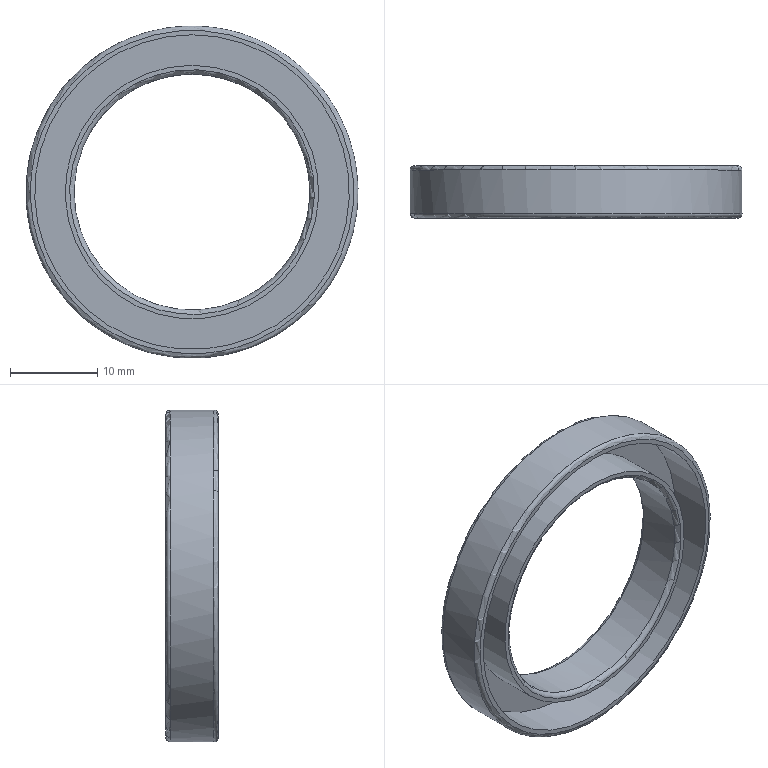Part | STEP file | BK-20_id1234_x_t | 1 solid | 12 faces | box 38 x 6 x 38 mm | volume 1518 mm3 | plane 4 | cylinder 4 | torus 4 | commonest cylinder face diameters 27 x1 29 x1 36 x1 38 x1